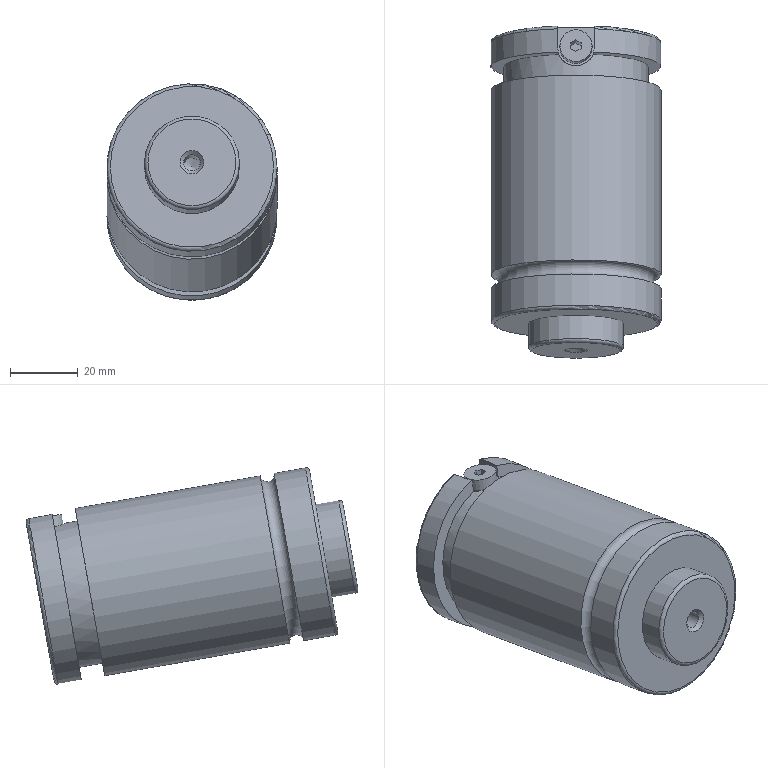Part | NX | features 1 2 | 1 solid | 34 faces | box 50.2 x 97.948 x 63.881 mm | volume 167121 mm3 | plane 16 | cylinder 10 | torus 4 | cone 4 | commonest cylinder face diameters 50.2 x3 6.6 x2 4.9 x1 9.5 x1 11 x1 28 x1
STEP:
#1=CARTESIAN_POINT('',(678.6,-1061.001,-253.867));
#2=VERTEX_POINT('',#1);
#3=CARTESIAN_POINT('',(653.5,-1061.001,-253.867));
#4=DIRECTION('',(0.,-0.9848,0.1736));
#5=DIRECTION('',(1.,0.,0.));
#6=AXIS2_PLACEMENT_3D('',#3,#4,#5);
#7=CIRCLE('',#6,25.1);
#8=EDGE_CURVE('',#2,#2,#7,.T.);
#9=ORIENTED_EDGE('',*,*,#8,.T.);
#10=EDGE_LOOP('',(#9));
#11=FACE_BOUND('',#10,.T.);
#12=CARTESIAN_POINT('',(678.6,-1065.137,-253.138));
#13=VERTEX_POINT('',#12);
#14=CARTESIAN_POINT('',(653.5,-1065.137,-253.138));
#15=DIRECTION('',(0.,-0.9848,0.1736));
#16=DIRECTION('',(1.,0.,0.));
#17=AXIS2_PLACEMENT_3D('',#14,#15,#16);
#18=CIRCLE('',#17,25.1);
#19=EDGE_CURVE('',#13,#13,#18,.T.);
#20=ORIENTED_EDGE('',*,*,#19,.F.);
#21=EDGE_LOOP('',(#20));
#22=FACE_BOUND('',#21,.T.);
#23=CARTESIAN_POINT('',(653.5,-1063.069,-253.502));
#24=DIRECTION('',(0.,-0.9848,0.1736));
#25=DIRECTION('',(0.,-0.1736,-0.9848));
#26=AXIS2_PLACEMENT_3D('',#23,#24,#25);
#27=TOROIDAL_SURFACE('',#26,25.1,2.1);
#28=ADVANCED_FACE('',(#11,#22),#27,.F.);
#29=CARTESIAN_POINT('',(678.6,-1074.394,-251.505));
#30=VERTEX_POINT('',#29);
#31=CARTESIAN_POINT('',(653.5,-1074.394,-251.505));
#32=DIRECTION('',(0.,-0.9848,0.1736));
#33=DIRECTION('',(1.,0.,0.));
#34=AXIS2_PLACEMENT_3D('',#31,#32,#33);
#35=CIRCLE('',#34,25.1);
#36=EDGE_CURVE('',#30,#30,#35,.T.);
#37=ORIENTED_EDGE('',*,*,#36,.T.);
#38=EDGE_LOOP('',(#37));
#39=FACE_BOUND('',#38,.T.);
#40=CARTESIAN_POINT('',(677.6,-1075.379,-251.332));
#41=VERTEX_POINT('',#40);
#42=CARTESIAN_POINT('',(653.5,-1075.379,-251.332));
#43=DIRECTION('',(0.,-0.9848,0.1736));
#44=DIRECTION('',(1.,0.,0.));
#45=AXIS2_PLACEMENT_3D('',#42,#43,#44);
#46=CIRCLE('',#45,24.1);
#47=EDGE_CURVE('',#41,#41,#46,.T.);
#48=ORIENTED_EDGE('',*,*,#47,.F.);
#49=EDGE_LOOP('',(#48));
#50=FACE_BOUND('',#49,.T.);
#51=CARTESIAN_POINT('',(653.5,-1074.394,-251.505));
#52=DIRECTION('',(0.,-0.9848,0.1736));
#53=DIRECTION('',(0.,-0.1736,-0.9848));
#54=AXIS2_PLACEMENT_3D('',#51,#52,#53);
#55=TOROIDAL_SURFACE('',#54,24.1,1.);
#56=ADVANCED_FACE('',(#39,#50),#55,.T.);
#57=ORIENTED_EDGE('',*,*,#19,.T.);
#58=EDGE_LOOP('',(#57));
#59=FACE_BOUND('',#58,.T.);
#60=ORIENTED_EDGE('',*,*,#36,.F.);
#61=EDGE_LOOP('',(#60));
#62=FACE_BOUND('',#61,.T.);
#63=CARTESIAN_POINT('',(653.5,-1069.766,-252.321));
#64=DIRECTION('',(0.,0.9848,-0.1736));
#65=DIRECTION('',(0.,0.1736,0.9848));
#66=AXIS2_PLACEMENT_3D('',#63,#64,#65);
#67=CYLINDRICAL_SURFACE('',#66,25.1);
#68=ADVANCED_FACE('',(#59,#62),#67,.T.);
#69=CARTESIAN_POINT('',(678.6,-1006.442,-263.487));
#70=VERTEX_POINT('',#69);
#71=CARTESIAN_POINT('',(653.5,-1006.442,-263.487));
#72=DIRECTION('',(0.,-0.9848,0.1736));
#73=DIRECTION('',(1.,0.,0.));
#74=AXIS2_PLACEMENT_3D('',#71,#72,#73);
#75=CIRCLE('',#74,25.1);
#76=EDGE_CURVE('',#70,#70,#75,.T.);
#77=ORIENTED_EDGE('',*,*,#76,.T.);
#78=EDGE_LOOP('',(#77));
#79=FACE_BOUND('',#78,.T.);
#80=ORIENTED_EDGE('',*,*,#8,.F.);
#81=EDGE_LOOP('',(#80));
#82=FACE_BOUND('',#81,.T.);
#83=CARTESIAN_POINT('',(653.5,-1026.828,-259.892));
#84=DIRECTION('',(0.,0.9848,-0.1736));
#85=DIRECTION('',(0.,0.1736,0.9848));
#86=AXIS2_PLACEMENT_3D('',#83,#84,#85);
#87=CYLINDRICAL_SURFACE('',#86,25.1);
#88=ADVANCED_FACE('',(#79,#82),#87,.T.);
#89=CARTESIAN_POINT('',(674.8,-1006.442,-263.487));
#90=VERTEX_POINT('',#89);
#91=CARTESIAN_POINT('',(653.5,-1006.442,-263.487));
#92=DIRECTION('',(0.,-0.9848,0.1736));
#93=DIRECTION('',(1.,0.,0.));
#94=AXIS2_PLACEMENT_3D('',#91,#92,#93);
#95=CIRCLE('',#94,21.3);
#96=EDGE_CURVE('',#90,#90,#95,.T.);
#97=ORIENTED_EDGE('',*,*,#96,.F.);
#98=EDGE_LOOP('',(#97));
#99=FACE_BOUND('',#98,.T.);
#100=CARTESIAN_POINT('',(648.377,-995.959,-244.342));
#101=VERTEX_POINT('',#100);
#102=CARTESIAN_POINT('',(658.623,-995.959,-244.342));
#103=VERTEX_POINT('',#102);
#104=CARTESIAN_POINT('',(653.5,-999.549,-264.702));
#105=DIRECTION('',(0.,-0.9848,0.1736));
#106=DIRECTION('',(1.,0.,0.));
#107=AXIS2_PLACEMENT_3D('',#104,#105,#106);
#108=CIRCLE('',#107,21.3);
#109=EDGE_CURVE('',#101,#103,#108,.T.);
#110=ORIENTED_EDGE('',*,*,#109,.T.);
#111=CARTESIAN_POINT('',(658.623,-995.959,-244.342));
#112=CARTESIAN_POINT('',(658.22,-996.96,-244.064));
#113=CARTESIAN_POINT('',(656.808,-998.646,-243.43));
#114=CARTESIAN_POINT('',(653.504,-999.621,-242.963));
#115=CARTESIAN_POINT('',(650.195,-998.65,-243.429));
#116=CARTESIAN_POINT('',(648.78,-996.96,-244.064));
#117=CARTESIAN_POINT('',(648.377,-995.959,-244.342));
#118=B_SPLINE_CURVE_WITH_KNOTS('',3,(#111,#112,#113,#114,#115,#116,#117),.UNSPECIFIED.,.F.,.F.,(4,1,1,1,4),(0.,0.003296,0.006593,0.009889,0.01319),.UNSPECIFIED.);
#119=EDGE_CURVE('',#103,#101,#118,.T.);
#120=ORIENTED_EDGE('',*,*,#119,.T.);
#121=EDGE_LOOP('',(#110,#120));
#122=FACE_BOUND('',#121,.T.);
#123=CARTESIAN_POINT('',(653.5,-1002.996,-264.095));
#124=DIRECTION('',(0.,0.9848,-0.1736));
#125=DIRECTION('',(0.,0.1736,0.9848));
#126=AXIS2_PLACEMENT_3D('',#123,#124,#125);
#127=CYLINDRICAL_SURFACE('',#126,21.3);
#128=ADVANCED_FACE('',(#99,#122),#127,.T.);
#129=CARTESIAN_POINT('',(667.5,-1082.273,-250.116));
#130=VERTEX_POINT('',#129);
#131=CARTESIAN_POINT('',(653.5,-1082.273,-250.116));
#132=DIRECTION('',(0.,-0.9848,0.1736));
#133=DIRECTION('',(1.,0.,0.));
#134=AXIS2_PLACEMENT_3D('',#131,#132,#133);
#135=CIRCLE('',#134,14.);
#136=EDGE_CURVE('',#130,#130,#135,.T.);
#137=ORIENTED_EDGE('',*,*,#136,.T.);
#138=EDGE_LOOP('',(#137));
#139=FACE_BOUND('',#138,.T.);
#140=CARTESIAN_POINT('',(666.5,-1083.257,-249.942));
#141=VERTEX_POINT('',#140);
#142=CARTESIAN_POINT('',(653.5,-1083.257,-249.942));
#143=DIRECTION('',(0.,-0.9848,0.1736));
#144=DIRECTION('',(1.,0.,0.));
#145=AXIS2_PLACEMENT_3D('',#142,#143,#144);
#146=CIRCLE('',#145,13.);
#147=EDGE_CURVE('',#141,#141,#146,.T.);
#148=ORIENTED_EDGE('',*,*,#147,.F.);
#149=EDGE_LOOP('',(#148));
#150=FACE_BOUND('',#149,.T.);
#151=CARTESIAN_POINT('',(653.5,-1082.273,-250.116));
#152=DIRECTION('',(0.,-0.9848,0.1736));
#153=DIRECTION('',(0.,-0.1736,-0.9848));
#154=AXIS2_PLACEMENT_3D('',#151,#152,#153);
#155=TOROIDAL_SURFACE('',#154,13.,1.);
#156=ADVANCED_FACE('',(#139,#150),#155,.T.);
#157=CARTESIAN_POINT('',(667.5,-1075.379,-251.332));
#158=VERTEX_POINT('',#157);
#159=CARTESIAN_POINT('',(653.5,-1075.379,-251.332));
#160=DIRECTION('',(0.,0.9848,-0.1736));
#161=DIRECTION('',(1.,0.,0.));
#162=AXIS2_PLACEMENT_3D('',#159,#160,#161);
#163=CIRCLE('',#162,14.);
#164=EDGE_CURVE('',#158,#158,#163,.T.);
#165=ORIENTED_EDGE('',*,*,#164,.F.);
#166=EDGE_LOOP('',(#165));
#167=FACE_BOUND('',#166,.T.);
#168=ORIENTED_EDGE('',*,*,#136,.F.);
#169=EDGE_LOOP('',(#168));
#170=FACE_BOUND('',#169,.T.);
#171=CARTESIAN_POINT('',(653.5,-1078.826,-250.724));
#172=DIRECTION('',(0.,0.9848,-0.1736));
#173=DIRECTION('',(0.,0.1736,0.9848));
#174=AXIS2_PLACEMENT_3D('',#171,#172,#173);
#175=CYLINDRICAL_SURFACE('',#174,14.);
#176=ADVANCED_FACE('',(#167,#170),#175,.T.);
#177=CARTESIAN_POINT('',(660.2,-991.67,-266.092));
#178=VERTEX_POINT('',#177);
#179=CARTESIAN_POINT('',(663.5,-991.67,-266.092));
#180=DIRECTION('',(0.,-0.9848,0.1736));
#181=DIRECTION('',(-1.,0.,0.));
#182=AXIS2_PLACEMENT_3D('',#179,#180,#181);
#183=CIRCLE('',#182,3.3);
#184=EDGE_CURVE('',#178,#178,#183,.T.);
#185=ORIENTED_EDGE('',*,*,#184,.F.);
#186=EDGE_LOOP('',(#185));
#187=FACE_BOUND('',#186,.T.);
#188=CARTESIAN_POINT('',(660.2,-1002.7,-264.147));
#189=VERTEX_POINT('',#188);
#190=CARTESIAN_POINT('',(663.5,-1002.7,-264.147));
#191=DIRECTION('',(0.,0.9848,-0.1736));
#192=DIRECTION('',(-1.,0.,0.));
#193=AXIS2_PLACEMENT_3D('',#190,#191,#192);
#194=CIRCLE('',#193,3.3);
#195=EDGE_CURVE('',#189,#189,#194,.T.);
#196=ORIENTED_EDGE('',*,*,#195,.F.);
#197=EDGE_LOOP('',(#196));
#198=FACE_BOUND('',#197,.T.);
#199=CARTESIAN_POINT('',(663.5,-997.185,-265.119));
#200=DIRECTION('',(0.,-0.9848,0.1736));
#201=DIRECTION('',(0.,-0.1736,-0.9848));
#202=AXIS2_PLACEMENT_3D('',#199,#200,#201);
#203=CYLINDRICAL_SURFACE('',#202,3.3);
#204=ADVANCED_FACE('',(#187,#198),#203,.F.);
#205=ORIENTED_EDGE('',*,*,#195,.T.);
#206=EDGE_LOOP('',(#205));
#207=FACE_BOUND('',#206,.T.);
#208=CARTESIAN_POINT('',(663.5,-1000.041,-264.616));
#209=VERTEX_POINT('',#208);
#210=VERTEX_LOOP('',#209);
#211=FACE_BOUND('',#210,.T.);
#212=CARTESIAN_POINT('',(663.5,-1001.371,-264.381));
#213=DIRECTION('',(0.,-0.9848,0.1736));
#214=DIRECTION('',(0.,-0.1736,-0.9848));
#215=AXIS2_PLACEMENT_3D('',#212,#213,#214);
#216=CONICAL_SURFACE('',#215,1.65,0.8851);
#217=ADVANCED_FACE('',(#207,#211),#216,.T.);
#218=CARTESIAN_POINT('',(657.,-1083.257,-249.942));
#219=VERTEX_POINT('',#218);
#220=CARTESIAN_POINT('',(653.5,-1083.257,-249.942));
#221=DIRECTION('',(0.,0.9848,-0.1736));
#222=DIRECTION('',(1.,0.,0.));
#223=AXIS2_PLACEMENT_3D('',#220,#221,#222);
#224=CIRCLE('',#223,3.5);
#225=EDGE_CURVE('',#219,#219,#224,.T.);
#226=ORIENTED_EDGE('',*,*,#225,.F.);
#227=EDGE_LOOP('',(#226));
#228=FACE_BOUND('',#227,.T.);
#229=CARTESIAN_POINT('',(655.95,-1082.223,-250.125));
#230=VERTEX_POINT('',#229);
#231=CARTESIAN_POINT('',(653.5,-1082.223,-250.125));
#232=DIRECTION('',(0.,-0.9848,0.1736));
#233=DIRECTION('',(1.,0.,0.));
#234=AXIS2_PLACEMENT_3D('',#231,#232,#233);
#235=CIRCLE('',#234,2.45);
#236=EDGE_CURVE('',#230,#230,#235,.T.);
#237=ORIENTED_EDGE('',*,*,#236,.F.);
#238=EDGE_LOOP('',(#237));
#239=FACE_BOUND('',#238,.T.);
#240=CARTESIAN_POINT('',(653.5,-1082.74,-250.034));
#241=DIRECTION('',(0.,-0.9848,0.1736));
#242=DIRECTION('',(0.,-0.1736,-0.9848));
#243=AXIS2_PLACEMENT_3D('',#240,#241,#242);
#244=CONICAL_SURFACE('',#243,2.975,0.7854);
#245=ADVANCED_FACE('',(#228,#239),#244,.F.);
#246=ORIENTED_EDGE('',*,*,#236,.T.);
#247=EDGE_LOOP('',(#246));
#248=FACE_BOUND('',#247,.T.);
#249=CARTESIAN_POINT('',(655.95,-1076.856,-251.071));
#250=VERTEX_POINT('',#249);
#251=CARTESIAN_POINT('',(653.5,-1076.856,-251.071));
#252=DIRECTION('',(0.,-0.9848,0.1736));
#253=DIRECTION('',(1.,0.,0.));
#254=AXIS2_PLACEMENT_3D('',#251,#252,#253);
#255=CIRCLE('',#254,2.45);
#256=EDGE_CURVE('',#250,#250,#255,.T.);
#257=ORIENTED_EDGE('',*,*,#256,.F.);
#258=EDGE_LOOP('',(#257));
#259=FACE_BOUND('',#258,.T.);
#260=CARTESIAN_POINT('',(653.5,-1079.54,-250.598));
#261=DIRECTION('',(0.,0.9848,-0.1736));
#262=DIRECTION('',(0.,0.1736,0.9848));
#263=AXIS2_PLACEMENT_3D('',#260,#261,#262);
#264=CYLINDRICAL_SURFACE('',#263,2.45);
#265=ADVANCED_FACE('',(#248,#259),#264,.F.);
#266=CARTESIAN_POINT('',(653.5,-1075.871,-251.245));
#267=VERTEX_POINT('',#266);
#268=VERTEX_LOOP('',#267);
#269=FACE_BOUND('',#268,.T.);
#270=ORIENTED_EDGE('',*,*,#256,.T.);
#271=EDGE_LOOP('',(#270));
#272=FACE_BOUND('',#271,.T.);
#273=CARTESIAN_POINT('',(653.5,-1076.364,-251.158));
#274=DIRECTION('',(0.,-0.9848,0.1736));
#275=DIRECTION('',(0.,-0.1736,-0.9848));
#276=AXIS2_PLACEMENT_3D('',#273,#274,#275);
#277=CONICAL_SURFACE('',#276,1.225,1.183);
#278=ADVANCED_FACE('',(#269,#272),#277,.F.);
#279=CARTESIAN_POINT('',(643.5,-1000.041,-264.616));
#280=VERTEX_POINT('',#279);
#281=VERTEX_LOOP('',#280);
#282=FACE_BOUND('',#281,.T.);
#283=CARTESIAN_POINT('',(646.8,-1002.7,-264.147));
#284=VERTEX_POINT('',#283);
#285=CARTESIAN_POINT('',(643.5,-1002.7,-264.147));
#286=DIRECTION('',(0.,-0.9848,0.1736));
#287=DIRECTION('',(1.,0.,0.));
#288=AXIS2_PLACEMENT_3D('',#285,#286,#287);
#289=CIRCLE('',#288,3.3);
#290=EDGE_CURVE('',#284,#284,#289,.T.);
#291=ORIENTED_EDGE('',*,*,#290,.F.);
#292=EDGE_LOOP('',(#291));
#293=FACE_BOUND('',#292,.T.);
#294=CARTESIAN_POINT('',(643.5,-1001.371,-264.381));
#295=DIRECTION('',(0.,-0.9848,0.1736));
#296=DIRECTION('',(0.,-0.1736,-0.9848));
#297=AXIS2_PLACEMENT_3D('',#294,#295,#296);
#298=CONICAL_SURFACE('',#297,1.65,0.8851);
#299=ADVANCED_FACE('',(#282,#293),#298,.T.);
#300=ORIENTED_EDGE('',*,*,#290,.T.);
#301=EDGE_LOOP('',(#300));
#302=FACE_BOUND('',#301,.T.);
#303=CARTESIAN_POINT('',(646.8,-991.67,-266.092));
#304=VERTEX_POINT('',#303);
#305=CARTESIAN_POINT('',(643.5,-991.67,-266.092));
#306=DIRECTION('',(0.,-0.9848,0.1736));
#307=DIRECTION('',(1.,0.,0.));
#308=AXIS2_PLACEMENT_3D('',#305,#306,#307);
#309=CIRCLE('',#308,3.3);
#310=EDGE_CURVE('',#304,#304,#309,.T.);
#311=ORIENTED_EDGE('',*,*,#310,.F.);
#312=EDGE_LOOP('',(#311));
#313=FACE_BOUND('',#312,.T.);
#314=CARTESIAN_POINT('',(643.5,-997.185,-265.119));
#315=DIRECTION('',(0.,0.9848,-0.1736));
#316=DIRECTION('',(0.,0.1736,0.9848));
#317=AXIS2_PLACEMENT_3D('',#314,#315,#316);
#318=CYLINDRICAL_SURFACE('',#317,3.3);
#319=ADVANCED_FACE('',(#302,#313),#318,.F.);
#320=CARTESIAN_POINT('',(648.,-988.403,-241.8));
#321=VERTEX_POINT('',#320);
#322=CARTESIAN_POINT('',(659.,-988.403,-241.8));
#323=VERTEX_POINT('',#322);
#324=CARTESIAN_POINT('',(653.5,-992.655,-265.918));
#325=DIRECTION('',(0.,-0.9848,0.1736));
#326=DIRECTION('',(1.,0.,0.));
#327=AXIS2_PLACEMENT_3D('',#324,#325,#326);
#328=CIRCLE('',#327,25.1);
#329=EDGE_CURVE('',#321,#323,#328,.T.);
#330=ORIENTED_EDGE('',*,*,#329,.T.);
#331=CARTESIAN_POINT('',(659.,-993.327,-240.932));
#332=VERTEX_POINT('',#331);
#333=CARTESIAN_POINT('',(659.,-990.865,-241.366));
#334=DIRECTION('',(0.,-0.9848,0.1736));
#335=VECTOR('',#334,1000.);
#336=LINE('',#333,#335);
#337=EDGE_CURVE('',#323,#332,#336,.T.);
#338=ORIENTED_EDGE('',*,*,#337,.T.);
#339=CARTESIAN_POINT('',(658.623,-995.282,-240.504));
#340=VERTEX_POINT('',#339);
#341=CARTESIAN_POINT('',(659.,-993.327,-240.932));
#342=CARTESIAN_POINT('',(659.,-994.007,-240.812));
#343=CARTESIAN_POINT('',(658.874,-994.659,-240.667));
#344=CARTESIAN_POINT('',(658.623,-995.282,-240.504));
#345=B_SPLINE_CURVE_WITH_KNOTS('',3,(#341,#342,#343,#344),.UNSPECIFIED.,.F.,.F.,(4,4),(0.,0.002037),.UNSPECIFIED.);
#346=EDGE_CURVE('',#332,#340,#345,.T.);
#347=ORIENTED_EDGE('',*,*,#346,.T.);
#348=CARTESIAN_POINT('',(648.377,-995.282,-240.504));
#349=VERTEX_POINT('',#348);
#350=CARTESIAN_POINT('',(653.5,-999.549,-264.702));
#351=DIRECTION('',(0.,0.9848,-0.1736));
#352=DIRECTION('',(1.,0.,0.));
#353=AXIS2_PLACEMENT_3D('',#350,#351,#352);
#354=CIRCLE('',#353,25.1);
#355=EDGE_CURVE('',#340,#349,#354,.T.);
#356=ORIENTED_EDGE('',*,*,#355,.T.);
#357=CARTESIAN_POINT('',(648.,-993.327,-240.932));
#358=VERTEX_POINT('',#357);
#359=CARTESIAN_POINT('',(648.377,-995.282,-240.504));
#360=CARTESIAN_POINT('',(648.126,-994.659,-240.667));
#361=CARTESIAN_POINT('',(648.,-994.007,-240.812));
#362=CARTESIAN_POINT('',(648.,-993.327,-240.932));
#363=B_SPLINE_CURVE_WITH_KNOTS('',3,(#359,#360,#361,#362),.UNSPECIFIED.,.F.,.F.,(4,4),(0.,0.002037),.UNSPECIFIED.);
#364=EDGE_CURVE('',#349,#358,#363,.T.);
#365=ORIENTED_EDGE('',*,*,#364,.T.);
#366=CARTESIAN_POINT('',(648.,-990.865,-241.366));
#367=DIRECTION('',(0.,0.9848,-0.1736));
#368=VECTOR('',#367,1000.);
#369=LINE('',#366,#368);
#370=EDGE_CURVE('',#358,#321,#369,.T.);
#371=ORIENTED_EDGE('',*,*,#370,.T.);
#372=EDGE_LOOP('',(#330,#338,#347,#356,#365,#371));
#373=FACE_BOUND('',#372,.T.);
#374=CARTESIAN_POINT('',(653.5,-1026.828,-259.892));
#375=DIRECTION('',(0.,0.9848,-0.1736));
#376=DIRECTION('',(0.,0.1736,0.9848));
#377=AXIS2_PLACEMENT_3D('',#374,#375,#376);
#378=CYLINDRICAL_SURFACE('',#377,25.1);
#379=ADVANCED_FACE('',(#373),#378,.T.);
#380=CARTESIAN_POINT('',(659.,-987.596,-242.984));
#381=VERTEX_POINT('',#380);
#382=CARTESIAN_POINT('',(659.,-987.596,-242.984));
#383=CARTESIAN_POINT('',(659.,-987.503,-242.457));
#384=CARTESIAN_POINT('',(659.,-987.875,-241.893));
#385=CARTESIAN_POINT('',(659.,-988.403,-241.8));
#386=B_SPLINE_CURVE_WITH_KNOTS('',3,(#382,#383,#384,#385),.UNSPECIFIED.,.F.,.F.,(4,4),(0.,0.001583),.UNSPECIFIED.);
#387=EDGE_CURVE('',#381,#323,#386,.T.);
#388=ORIENTED_EDGE('',*,*,#387,.T.);
#389=ORIENTED_EDGE('',*,*,#329,.F.);
#390=CARTESIAN_POINT('',(648.,-987.596,-242.984));
#391=VERTEX_POINT('',#390);
#392=CARTESIAN_POINT('',(648.,-988.403,-241.8));
#393=CARTESIAN_POINT('',(648.,-987.875,-241.893));
#394=CARTESIAN_POINT('',(648.,-987.503,-242.457));
#395=CARTESIAN_POINT('',(648.,-987.596,-242.984));
#396=B_SPLINE_CURVE_WITH_KNOTS('',3,(#392,#393,#394,#395),.UNSPECIFIED.,.F.,.F.,(4,4),(0.,0.001583),.UNSPECIFIED.);
#397=EDGE_CURVE('',#321,#391,#396,.T.);
#398=ORIENTED_EDGE('',*,*,#397,.T.);
#399=CARTESIAN_POINT('',(653.5,-991.67,-266.092));
#400=DIRECTION('',(0.,-0.9848,0.1736));
#401=DIRECTION('',(1.,0.,0.));
#402=AXIS2_PLACEMENT_3D('',#399,#400,#401);
#403=CIRCLE('',#402,24.1);
#404=EDGE_CURVE('',#391,#381,#403,.T.);
#405=ORIENTED_EDGE('',*,*,#404,.T.);
#406=EDGE_LOOP('',(#388,#389,#398,#405));
#407=FACE_BOUND('',#406,.T.);
#408=CARTESIAN_POINT('',(653.5,-992.655,-265.918));
#409=DIRECTION('',(0.,-0.9848,0.1736));
#410=DIRECTION('',(0.,-0.1736,-0.9848));
#411=AXIS2_PLACEMENT_3D('',#408,#409,#410);
#412=TOROIDAL_SURFACE('',#411,24.1,1.);
#413=ADVANCED_FACE('',(#407),#412,.T.);
#414=CARTESIAN_POINT('',(658.25,-994.002,-244.763));
#415=VERTEX_POINT('',#414);
#416=CARTESIAN_POINT('',(653.5,-994.002,-244.763));
#417=DIRECTION('',(0.,-0.1736,-0.9848));
#418=DIRECTION('',(1.,0.,0.));
#419=AXIS2_PLACEMENT_3D('',#416,#417,#418);
#420=CIRCLE('',#419,4.75);
#421=EDGE_CURVE('',#415,#415,#420,.T.);
#422=ORIENTED_EDGE('',*,*,#421,.F.);
#423=EDGE_LOOP('',(#422));
#424=FACE_BOUND('',#423,.T.);
#425=CARTESIAN_POINT('',(658.25,-993.394,-241.316));
#426=VERTEX_POINT('',#425);
#427=CARTESIAN_POINT('',(653.5,-993.394,-241.316));
#428=DIRECTION('',(0.,-0.1736,-0.9848));
#429=DIRECTION('',(1.,0.,0.));
#430=AXIS2_PLACEMENT_3D('',#427,#428,#429);
#431=CIRCLE('',#430,4.75);
#432=EDGE_CURVE('',#426,#426,#431,.T.);
#433=ORIENTED_EDGE('',*,*,#432,.T.);
#434=EDGE_LOOP('',(#433));
#435=FACE_BOUND('',#434,.T.);
#436=CARTESIAN_POINT('',(653.5,-997.579,-265.05));
#437=DIRECTION('',(0.,-0.1736,-0.9848));
#438=DIRECTION('',(1.,0.,0.));
#439=AXIS2_PLACEMENT_3D('',#436,#437,#438);
#440=CYLINDRICAL_SURFACE('',#439,4.75);
#441=ADVANCED_FACE('',(#424,#435),#440,.T.);
#442=CARTESIAN_POINT('',(655.,-993.41,-246.39));
#443=VERTEX_POINT('',#442);
#444=CARTESIAN_POINT('',(653.5,-992.557,-246.541));
#445=VERTEX_POINT('',#444);
#446=CARTESIAN_POINT('',(655.,-993.41,-246.39));
#447=DIRECTION('',(-0.866,0.4924,-0.08682));
#448=VECTOR('',#447,1000.);
#449=LINE('',#446,#448);
#450=EDGE_CURVE('',#443,#445,#449,.T.);
#451=ORIENTED_EDGE('',*,*,#450,.F.);
#452=CARTESIAN_POINT('',(655.,-992.541,-241.466));
#453=VERTEX_POINT('',#452);
#454=CARTESIAN_POINT('',(655.,-992.541,-241.466));
#455=DIRECTION('',(0.,-0.1736,-0.9848));
#456=VECTOR('',#455,1000.);
#457=LINE('',#454,#456);
#458=EDGE_CURVE('',#453,#443,#457,.T.);
#459=ORIENTED_EDGE('',*,*,#458,.F.);
#460=CARTESIAN_POINT('',(653.5,-991.689,-241.617));
#461=VERTEX_POINT('',#460);
#462=CARTESIAN_POINT('',(653.326,-991.59,-241.634));
#463=DIRECTION('',(0.866,-0.4924,0.08682));
#464=VECTOR('',#463,1000.);
#465=LINE('',#462,#464);
#466=EDGE_CURVE('',#461,#453,#465,.T.);
#467=ORIENTED_EDGE('',*,*,#466,.F.);
#468=CARTESIAN_POINT('',(653.5,-991.689,-241.617));
#469=DIRECTION('',(0.,-0.1736,-0.9848));
#470=VECTOR('',#469,1000.);
#471=LINE('',#468,#470);
#472=EDGE_CURVE('',#461,#445,#471,.T.);
#473=ORIENTED_EDGE('',*,*,#472,.T.);
#474=EDGE_LOOP('',(#451,#459,#467,#473));
#475=FACE_BOUND('',#474,.T.);
#476=CARTESIAN_POINT('',(655.,-992.541,-241.466));
#477=DIRECTION('',(0.5,0.8529,-0.1504));
#478=DIRECTION('',(0.866,-0.4924,0.08682));
#479=AXIS2_PLACEMENT_3D('',#476,#477,#478);
#480=PLANE('',#479);
#481=ADVANCED_FACE('',(#475),#480,.F.);
#482=CARTESIAN_POINT('',(652.,-993.41,-246.39));
#483=VERTEX_POINT('',#482);
#484=CARTESIAN_POINT('',(653.5,-992.557,-246.541));
#485=DIRECTION('',(-0.866,-0.4924,0.08682));
#486=VECTOR('',#485,1000.);
#487=LINE('',#484,#486);
#488=EDGE_CURVE('',#445,#483,#487,.T.);
#489=ORIENTED_EDGE('',*,*,#488,.F.);
#490=ORIENTED_EDGE('',*,*,#472,.F.);
#491=CARTESIAN_POINT('',(652.,-992.541,-241.466));
#492=VERTEX_POINT('',#491);
#493=CARTESIAN_POINT('',(654.424,-991.163,-241.709));
#494=DIRECTION('',(0.866,0.4924,-0.08682));
#495=VECTOR('',#494,1000.);
#496=LINE('',#493,#495);
#497=EDGE_CURVE('',#492,#461,#496,.T.);
#498=ORIENTED_EDGE('',*,*,#497,.F.);
#499=CARTESIAN_POINT('',(652.,-992.541,-241.466));
#500=DIRECTION('',(0.,-0.1736,-0.9848));
#501=VECTOR('',#500,1000.);
#502=LINE('',#499,#501);
#503=EDGE_CURVE('',#492,#483,#502,.T.);
#504=ORIENTED_EDGE('',*,*,#503,.T.);
#505=EDGE_LOOP('',(#489,#490,#498,#504));
#506=FACE_BOUND('',#505,.T.);
#507=CARTESIAN_POINT('',(653.5,-991.689,-241.617));
#508=DIRECTION('',(-0.5,0.8529,-0.1504));
#509=DIRECTION('',(0.866,0.4924,-0.08682));
#510=AXIS2_PLACEMENT_3D('',#507,#508,#509);
#511=PLANE('',#510);
#512=ADVANCED_FACE('',(#506),#511,.F.);
#513=CARTESIAN_POINT('',(652.,-995.115,-246.09));
#514=VERTEX_POINT('',#513);
#515=CARTESIAN_POINT('',(652.,-993.41,-246.39));
#516=DIRECTION('',(0.,-0.9848,0.1736));
#517=VECTOR('',#516,1000.);
#518=LINE('',#515,#517);
#519=EDGE_CURVE('',#483,#514,#518,.T.);
#520=ORIENTED_EDGE('',*,*,#519,.F.);
#521=ORIENTED_EDGE('',*,*,#503,.F.);
#522=CARTESIAN_POINT('',(652.,-994.247,-241.166));
#523=VERTEX_POINT('',#522);
#524=CARTESIAN_POINT('',(652.,-990.013,-241.912));
#525=DIRECTION('',(0.,0.9848,-0.1736));
#526=VECTOR('',#525,1000.);
#527=LINE('',#524,#526);
#528=EDGE_CURVE('',#523,#492,#527,.T.);
#529=ORIENTED_EDGE('',*,*,#528,.F.);
#530=CARTESIAN_POINT('',(652.,-994.247,-241.166));
#531=DIRECTION('',(0.,-0.1736,-0.9848));
#532=VECTOR('',#531,1000.);
#533=LINE('',#530,#532);
#534=EDGE_CURVE('',#523,#514,#533,.T.);
#535=ORIENTED_EDGE('',*,*,#534,.T.);
#536=EDGE_LOOP('',(#520,#521,#529,#535));
#537=FACE_BOUND('',#536,.T.);
#538=CARTESIAN_POINT('',(652.,-992.541,-241.466));
#539=DIRECTION('',(-1.,0.,0.));
#540=DIRECTION('',(0.,-0.1736,-0.9848));
#541=AXIS2_PLACEMENT_3D('',#538,#539,#540);
#542=PLANE('',#541);
#543=ADVANCED_FACE('',(#537),#542,.F.);
#544=CARTESIAN_POINT('',(653.5,-995.968,-245.939));
#545=VERTEX_POINT('',#544);
#546=CARTESIAN_POINT('',(652.,-995.115,-246.09));
#547=DIRECTION('',(0.866,-0.4924,0.08682));
#548=VECTOR('',#547,1000.);
#549=LINE('',#546,#548);
#550=EDGE_CURVE('',#514,#545,#549,.T.);
#551=ORIENTED_EDGE('',*,*,#550,.F.);
#552=ORIENTED_EDGE('',*,*,#534,.F.);
#553=CARTESIAN_POINT('',(653.5,-995.1,-241.015));
#554=VERTEX_POINT('',#553);
#555=CARTESIAN_POINT('',(651.076,-993.722,-241.258));
#556=DIRECTION('',(-0.866,0.4924,-0.08682));
#557=VECTOR('',#556,1000.);
#558=LINE('',#555,#557);
#559=EDGE_CURVE('',#554,#523,#558,.T.);
#560=ORIENTED_EDGE('',*,*,#559,.F.);
#561=CARTESIAN_POINT('',(653.5,-995.1,-241.015));
#562=DIRECTION('',(0.,-0.1736,-0.9848));
#563=VECTOR('',#562,1000.);
#564=LINE('',#561,#563);
#565=EDGE_CURVE('',#554,#545,#564,.T.);
#566=ORIENTED_EDGE('',*,*,#565,.T.);
#567=EDGE_LOOP('',(#551,#552,#560,#566));
#568=FACE_BOUND('',#567,.T.);
#569=CARTESIAN_POINT('',(652.,-994.247,-241.166));
#570=DIRECTION('',(-0.5,-0.8529,0.1504));
#571=DIRECTION('',(-0.866,0.4924,-0.08682));
#572=AXIS2_PLACEMENT_3D('',#569,#570,#571);
#573=PLANE('',#572);
#574=ADVANCED_FACE('',(#568),#573,.F.);
#575=CARTESIAN_POINT('',(655.,-995.115,-246.09));
#576=VERTEX_POINT('',#575);
#577=CARTESIAN_POINT('',(653.5,-995.968,-245.939));
#578=DIRECTION('',(0.866,0.4924,-0.08682));
#579=VECTOR('',#578,1000.);
#580=LINE('',#577,#579);
#581=EDGE_CURVE('',#545,#576,#580,.T.);
#582=ORIENTED_EDGE('',*,*,#581,.F.);
#583=ORIENTED_EDGE('',*,*,#565,.F.);
#584=CARTESIAN_POINT('',(655.,-994.247,-241.166));
#585=VERTEX_POINT('',#584);
#586=CARTESIAN_POINT('',(655.174,-994.148,-241.183));
#587=DIRECTION('',(-0.866,-0.4924,0.08682));
#588=VECTOR('',#587,1000.);
#589=LINE('',#586,#588);
#590=EDGE_CURVE('',#585,#554,#589,.T.);
#591=ORIENTED_EDGE('',*,*,#590,.F.);
#592=CARTESIAN_POINT('',(655.,-994.247,-241.166));
#593=DIRECTION('',(0.,-0.1736,-0.9848));
#594=VECTOR('',#593,1000.);
#595=LINE('',#592,#594);
#596=EDGE_CURVE('',#585,#576,#595,.T.);
#597=ORIENTED_EDGE('',*,*,#596,.T.);
#598=EDGE_LOOP('',(#582,#583,#591,#597));
#599=FACE_BOUND('',#598,.T.);
#600=CARTESIAN_POINT('',(653.5,-995.1,-241.015));
#601=DIRECTION('',(0.5,-0.8529,0.1504));
#602=DIRECTION('',(-0.866,-0.4924,0.08682));
#603=AXIS2_PLACEMENT_3D('',#600,#601,#602);
#604=PLANE('',#603);
#605=ADVANCED_FACE('',(#599),#604,.F.);
#606=CARTESIAN_POINT('',(655.,-995.115,-246.09));
#607=DIRECTION('',(0.,0.9848,-0.1736));
#608=VECTOR('',#607,1000.);
#609=LINE('',#606,#608);
#610=EDGE_CURVE('',#576,#443,#609,.T.);
#611=ORIENTED_EDGE('',*,*,#610,.F.);
#612=ORIENTED_EDGE('',*,*,#596,.F.);
#613=CARTESIAN_POINT('',(655.,-990.866,-241.762));
#614=DIRECTION('',(0.,-0.9848,0.1736));
#615=VECTOR('',#614,1000.);
#616=LINE('',#613,#615);
#617=EDGE_CURVE('',#453,#585,#616,.T.);
#618=ORIENTED_EDGE('',*,*,#617,.F.);
#619=ORIENTED_EDGE('',*,*,#458,.T.);
#620=EDGE_LOOP('',(#611,#612,#618,#619));
#621=FACE_BOUND('',#620,.T.);
#622=CARTESIAN_POINT('',(655.,-994.247,-241.166));
#623=DIRECTION('',(1.,0.,0.));
#624=DIRECTION('',(0.,0.1736,0.9848));
#625=AXIS2_PLACEMENT_3D('',#622,#623,#624);
#626=PLANE('',#625);
#627=ADVANCED_FACE('',(#621),#626,.F.);
#628=ORIENTED_EDGE('',*,*,#450,.T.);
#629=ORIENTED_EDGE('',*,*,#488,.T.);
#630=ORIENTED_EDGE('',*,*,#519,.T.);
#631=ORIENTED_EDGE('',*,*,#550,.T.);
#632=ORIENTED_EDGE('',*,*,#581,.T.);
#633=ORIENTED_EDGE('',*,*,#610,.T.);
#634=EDGE_LOOP('',(#628,#629,#630,#631,#632,#633));
#635=FACE_BOUND('',#634,.T.);
#636=CARTESIAN_POINT('',(653.5,-994.263,-246.24));
#637=DIRECTION('',(0.,0.1736,0.9848));
#638=DIRECTION('',(-1.,0.,0.));
#639=AXIS2_PLACEMENT_3D('',#636,#637,#638);
#640=PLANE('',#639);
#641=ADVANCED_FACE('',(#635),#640,.T.);
#642=ORIENTED_EDGE('',*,*,#466,.T.);
#643=ORIENTED_EDGE('',*,*,#617,.T.);
#644=ORIENTED_EDGE('',*,*,#590,.T.);
#645=ORIENTED_EDGE('',*,*,#559,.T.);
#646=ORIENTED_EDGE('',*,*,#528,.T.);
#647=ORIENTED_EDGE('',*,*,#497,.T.);
#648=EDGE_LOOP('',(#642,#643,#644,#645,#646,#647));
#649=FACE_BOUND('',#648,.T.);
#650=ORIENTED_EDGE('',*,*,#432,.F.);
#651=EDGE_LOOP('',(#650));
#652=FACE_BOUND('',#651,.T.);
#653=CARTESIAN_POINT('',(653.5,-987.485,-242.358));
#654=DIRECTION('',(0.,-0.1736,-0.9848));
#655=DIRECTION('',(1.,0.,0.));
#656=AXIS2_PLACEMENT_3D('',#653,#654,#655);
#657=PLANE('',#656);
#658=ADVANCED_FACE('',(#649,#652),#657,.F.);
#659=ORIENTED_EDGE('',*,*,#370,.F.);
#660=CARTESIAN_POINT('',(648.,-994.002,-244.763));
#661=VERTEX_POINT('',#660);
#662=CARTESIAN_POINT('',(648.,-993.221,-240.331));
#663=DIRECTION('',(0.,-0.1736,-0.9848));
#664=VECTOR('',#663,1000.);
#665=LINE('',#662,#664);
#666=EDGE_CURVE('',#358,#661,#665,.T.);
#667=ORIENTED_EDGE('',*,*,#666,.T.);
#668=CARTESIAN_POINT('',(648.,-988.093,-245.805));
#669=VERTEX_POINT('',#668);
#670=CARTESIAN_POINT('',(648.,-994.002,-244.763));
#671=DIRECTION('',(0.,-0.9848,0.1736));
#672=VECTOR('',#671,1000.);
#673=LINE('',#670,#672);
#674=EDGE_CURVE('',#669,#661,#673,.T.);
#675=ORIENTED_EDGE('',*,*,#674,.F.);
#676=CARTESIAN_POINT('',(648.,-989.491,-253.732));
#677=DIRECTION('',(0.,-0.1736,-0.9848));
#678=VECTOR('',#677,1000.);
#679=LINE('',#676,#678);
#680=EDGE_CURVE('',#391,#669,#679,.T.);
#681=ORIENTED_EDGE('',*,*,#680,.F.);
#682=ORIENTED_EDGE('',*,*,#397,.F.);
#683=EDGE_LOOP('',(#659,#667,#675,#681,#682));
#684=FACE_BOUND('',#683,.T.);
#685=CARTESIAN_POINT('',(648.,-987.312,-241.373));
#686=DIRECTION('',(-1.,0.,0.));
#687=DIRECTION('',(0.,-0.1736,-0.9848));
#688=AXIS2_PLACEMENT_3D('',#685,#686,#687);
#689=PLANE('',#688);
#690=ADVANCED_FACE('',(#684),#689,.F.);
#691=ORIENTED_EDGE('',*,*,#364,.F.);
#692=CARTESIAN_POINT('',(648.377,-995.581,-242.2));
#693=DIRECTION('',(0.,0.1736,0.9848));
#694=VECTOR('',#693,1000.);
#695=LINE('',#692,#694);
#696=EDGE_CURVE('',#101,#349,#695,.T.);
#697=ORIENTED_EDGE('',*,*,#696,.F.);
#698=ORIENTED_EDGE('',*,*,#119,.F.);
#699=CARTESIAN_POINT('',(658.623,-995.581,-242.2));
#700=DIRECTION('',(0.,-0.1736,-0.9848));
#701=VECTOR('',#700,1000.);
#702=LINE('',#699,#701);
#703=EDGE_CURVE('',#340,#103,#702,.T.);
#704=ORIENTED_EDGE('',*,*,#703,.F.);
#705=ORIENTED_EDGE('',*,*,#346,.F.);
#706=CARTESIAN_POINT('',(659.,-994.002,-244.763));
#707=VERTEX_POINT('',#706);
#708=CARTESIAN_POINT('',(659.,-993.221,-240.331));
#709=DIRECTION('',(0.,-0.1736,-0.9848));
#710=VECTOR('',#709,1000.);
#711=LINE('',#708,#710);
#712=EDGE_CURVE('',#332,#707,#711,.T.);
#713=ORIENTED_EDGE('',*,*,#712,.T.);
#714=CARTESIAN_POINT('',(653.5,-994.002,-244.763));
#715=DIRECTION('',(0.,0.1736,0.9848));
#716=DIRECTION('',(1.,0.,0.));
#717=AXIS2_PLACEMENT_3D('',#714,#715,#716);
#718=CIRCLE('',#717,5.5);
#719=EDGE_CURVE('',#661,#707,#718,.T.);
#720=ORIENTED_EDGE('',*,*,#719,.F.);
#721=ORIENTED_EDGE('',*,*,#666,.F.);
#722=EDGE_LOOP('',(#691,#697,#698,#704,#705,#713,#720,#721));
#723=FACE_BOUND('',#722,.T.);
#724=CARTESIAN_POINT('',(653.5,-993.221,-240.331));
#725=DIRECTION('',(0.,0.1736,0.9848));
#726=DIRECTION('',(-1.,0.,0.));
#727=AXIS2_PLACEMENT_3D('',#724,#725,#726);
#728=CYLINDRICAL_SURFACE('',#727,5.5);
#729=ADVANCED_FACE('',(#723),#728,.F.);
#730=ORIENTED_EDGE('',*,*,#337,.F.);
#731=ORIENTED_EDGE('',*,*,#387,.F.);
#732=CARTESIAN_POINT('',(659.,-988.093,-245.805));
#733=VERTEX_POINT('',#732);
#734=CARTESIAN_POINT('',(659.,-989.491,-253.732));
#735=DIRECTION('',(0.,0.1736,0.9848));
#736=VECTOR('',#735,1000.);
#737=LINE('',#734,#736);
#738=EDGE_CURVE('',#733,#381,#737,.T.);
#739=ORIENTED_EDGE('',*,*,#738,.F.);
#740=CARTESIAN_POINT('',(659.,-988.093,-245.805));
#741=DIRECTION('',(0.,0.9848,-0.1736));
#742=VECTOR('',#741,1000.);
#743=LINE('',#740,#742);
#744=EDGE_CURVE('',#707,#733,#743,.T.);
#745=ORIENTED_EDGE('',*,*,#744,.F.);
#746=ORIENTED_EDGE('',*,*,#712,.F.);
#747=EDGE_LOOP('',(#730,#731,#739,#745,#746));
#748=FACE_BOUND('',#747,.T.);
#749=CARTESIAN_POINT('',(659.,-993.221,-240.331));
#750=DIRECTION('',(1.,0.,0.));
#751=DIRECTION('',(0.,0.1736,0.9848));
#752=AXIS2_PLACEMENT_3D('',#749,#750,#751);
#753=PLANE('',#752);
#754=ADVANCED_FACE('',(#748),#753,.F.);
#755=ORIENTED_EDGE('',*,*,#421,.T.);
#756=EDGE_LOOP('',(#755));
#757=FACE_BOUND('',#756,.T.);
#758=ORIENTED_EDGE('',*,*,#674,.T.);
#759=ORIENTED_EDGE('',*,*,#719,.T.);
#760=ORIENTED_EDGE('',*,*,#744,.T.);
#761=CARTESIAN_POINT('',(659.525,-988.093,-245.805));
#762=DIRECTION('',(1.,0.,0.));
#763=VECTOR('',#762,1000.);
#764=LINE('',#761,#763);
#765=EDGE_CURVE('',#669,#733,#764,.T.);
#766=ORIENTED_EDGE('',*,*,#765,.F.);
#767=EDGE_LOOP('',(#758,#759,#760,#766));
#768=FACE_BOUND('',#767,.T.);
#769=CARTESIAN_POINT('',(653.5,-988.093,-245.805));
#770=DIRECTION('',(0.,-0.1736,-0.9848));
#771=DIRECTION('',(1.,0.,0.));
#772=AXIS2_PLACEMENT_3D('',#769,#770,#771);
#773=PLANE('',#772);
#774=ADVANCED_FACE('',(#757,#768),#773,.F.);
#775=ORIENTED_EDGE('',*,*,#696,.T.);
#776=ORIENTED_EDGE('',*,*,#355,.F.);
#777=ORIENTED_EDGE('',*,*,#703,.T.);
#778=ORIENTED_EDGE('',*,*,#109,.F.);
#779=EDGE_LOOP('',(#775,#776,#777,#778));
#780=FACE_BOUND('',#779,.T.);
#781=CARTESIAN_POINT('',(676.8,-999.549,-264.702));
#782=DIRECTION('',(0.,0.9848,-0.1736));
#783=DIRECTION('',(0.,0.1736,0.9848));
#784=AXIS2_PLACEMENT_3D('',#781,#782,#783);
#785=PLANE('',#784);
#786=ADVANCED_FACE('',(#780),#785,.F.);
#787=ORIENTED_EDGE('',*,*,#680,.T.);
#788=ORIENTED_EDGE('',*,*,#765,.T.);
#789=ORIENTED_EDGE('',*,*,#738,.T.);
#790=ORIENTED_EDGE('',*,*,#404,.F.);
#791=EDGE_LOOP('',(#787,#788,#789,#790));
#792=FACE_BOUND('',#791,.T.);
#793=ORIENTED_EDGE('',*,*,#184,.T.);
#794=EDGE_LOOP('',(#793));
#795=FACE_BOUND('',#794,.T.);
#796=ORIENTED_EDGE('',*,*,#310,.T.);
#797=EDGE_LOOP('',(#796));
#798=FACE_BOUND('',#797,.T.);
#799=CARTESIAN_POINT('',(665.55,-991.67,-266.092));
#800=DIRECTION('',(0.,0.9848,-0.1736));
#801=DIRECTION('',(1.,0.,0.));
#802=AXIS2_PLACEMENT_3D('',#799,#800,#801);
#803=PLANE('',#802);
#804=ADVANCED_FACE('',(#792,#795,#798),#803,.T.);
#805=ORIENTED_EDGE('',*,*,#225,.T.);
#806=EDGE_LOOP('',(#805));
#807=FACE_BOUND('',#806,.T.);
#808=ORIENTED_EDGE('',*,*,#147,.T.);
#809=EDGE_LOOP('',(#808));
#810=FACE_BOUND('',#809,.T.);
#811=CARTESIAN_POINT('',(660.,-1083.257,-249.942));
#812=DIRECTION('',(0.,-0.9848,0.1736));
#813=DIRECTION('',(0.,-0.1736,-0.9848));
#814=AXIS2_PLACEMENT_3D('',#811,#812,#813);
#815=PLANE('',#814);
#816=ADVANCED_FACE('',(#807,#810),#815,.T.);
#817=ORIENTED_EDGE('',*,*,#76,.F.);
#818=EDGE_LOOP('',(#817));
#819=FACE_BOUND('',#818,.T.);
#820=ORIENTED_EDGE('',*,*,#96,.T.);
#821=EDGE_LOOP('',(#820));
#822=FACE_BOUND('',#821,.T.);
#823=CARTESIAN_POINT('',(676.8,-1006.442,-263.487));
#824=DIRECTION('',(0.,-0.9848,0.1736));
#825=DIRECTION('',(0.,-0.1736,-0.9848));
#826=AXIS2_PLACEMENT_3D('',#823,#824,#825);
#827=PLANE('',#826);
#828=ADVANCED_FACE('',(#819,#822),#827,.F.);
#829=ORIENTED_EDGE('',*,*,#164,.T.);
#830=EDGE_LOOP('',(#829));
#831=FACE_BOUND('',#830,.T.);
#832=ORIENTED_EDGE('',*,*,#47,.T.);
#833=EDGE_LOOP('',(#832));
#834=FACE_BOUND('',#833,.T.);
#835=CARTESIAN_POINT('',(665.55,-1075.379,-251.332));
#836=DIRECTION('',(0.,-0.9848,0.1736));
#837=DIRECTION('',(0.,-0.1736,-0.9848));
#838=AXIS2_PLACEMENT_3D('',#835,#836,#837);
#839=PLANE('',#838);
#840=ADVANCED_FACE('',(#831,#834),#839,.T.);
#841=CLOSED_SHELL('',(#28,#56,#68,#88,#128,#156,#176,#204,#217,#245,#265,#278,#299,#319,#379,#413,#441,#481,#512,#543,#574,#605,#627,#641,#658,#690,#729,#754,#774,#786,#804,#816,#828,#840));
#842=MANIFOLD_SOLID_BREP('',#841);
#843=(LENGTH_UNIT()NAMED_UNIT(*)SI_UNIT(.MILLI.,.METRE.));
#844=UNCERTAINTY_MEASURE_WITH_UNIT(LENGTH_MEASURE(0.0508),#843,'','');
#845=(NAMED_UNIT(*)PLANE_ANGLE_UNIT()SI_UNIT($,.RADIAN.));
#846=(NAMED_UNIT(*)SI_UNIT($,.STERADIAN.)SOLID_ANGLE_UNIT());
#847=(GEOMETRIC_REPRESENTATION_CONTEXT(3)GLOBAL_UNCERTAINTY_ASSIGNED_CONTEXT((#844))GLOBAL_UNIT_ASSIGNED_CONTEXT((#843,#845,#846))REPRESENTATION_CONTEXT('',''));
#848=ADVANCED_BREP_SHAPE_REPRESENTATION('',(#842),#847);